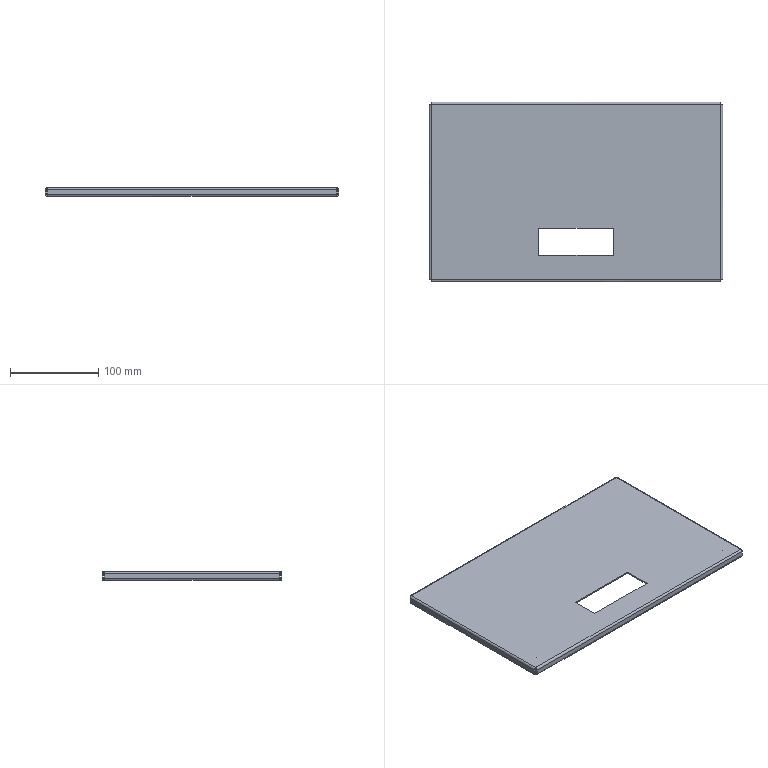Part | SolidWorks | features EdgeFlange 2, ICE 2, Cut 1, Fillet 1, FlatPattern 1, HoleWzd 1, SMBaseFlange 1, SheetMetal 1 | 1 solid | 102 faces | box 333 x 204 x 10 mm | volume 124436 mm3 | plane 54 | cylinder 28 | spline 16 | cone 4 | commonest cylinder face diameters 1.473 x8 4.473 x8 2.5 x4 4 x4 8.1 x4